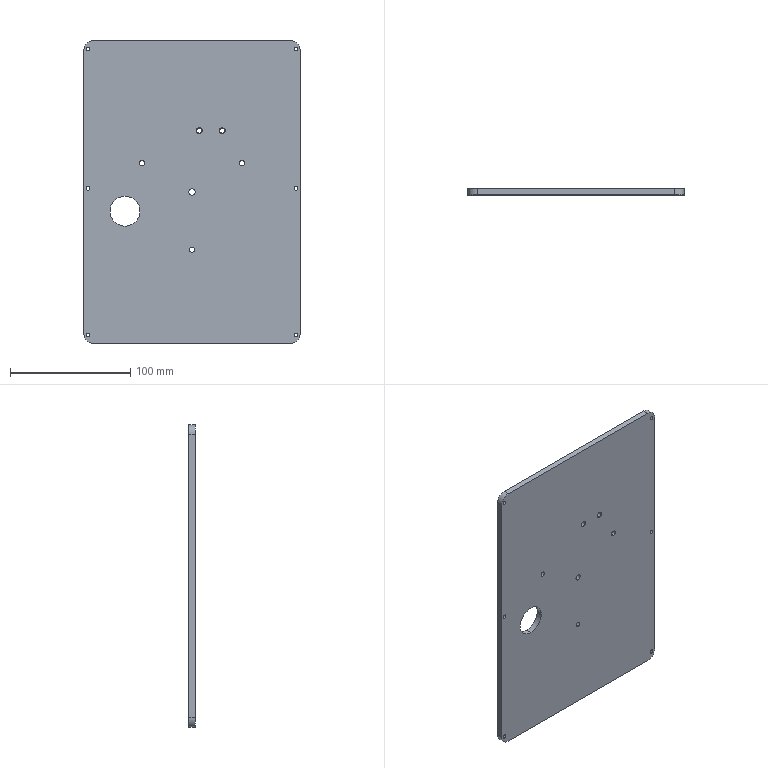Part | SolidWorks | features ICE 5, HoleWzd 2, Dome 1, Extrusion 1, Fillet 1 | 1 solid | 52 faces | box 180 x 5 x 252 mm | volume 223279 mm3 | cylinder 30 | cone 16 | plane 6 | commonest cylinder face diameters 3.2 x12 4.2 x10 16 x4 5.2 x2 25 x2